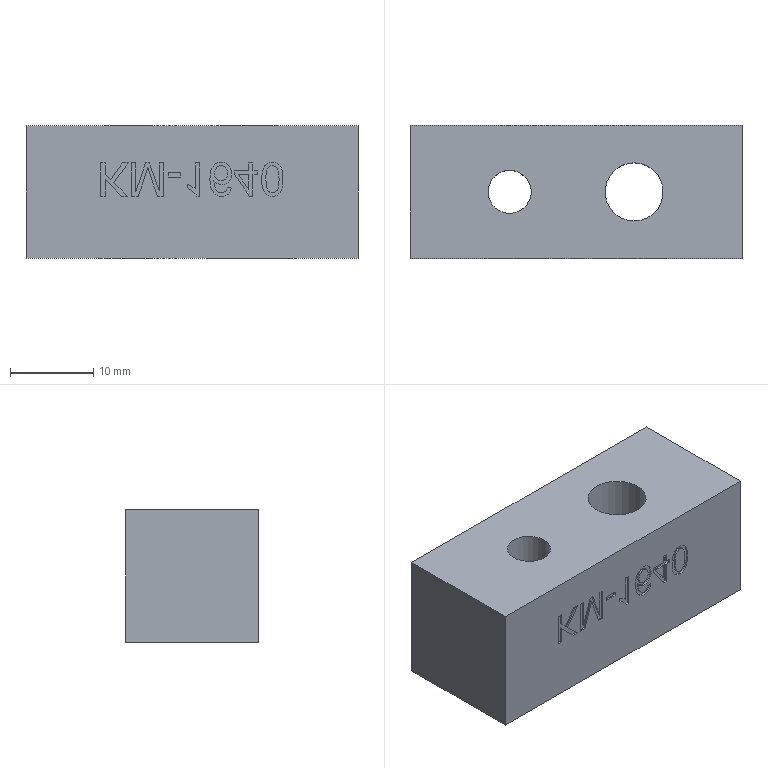Part | NX | features solid 2 | 1 solid | 83 faces | box 40 x 16 x 16 mm | volume 8723 mm3 | plane 65 | spline 14 | cylinder 4 | commonest cylinder face diameters 7 x2 5.2 x1 11 x1